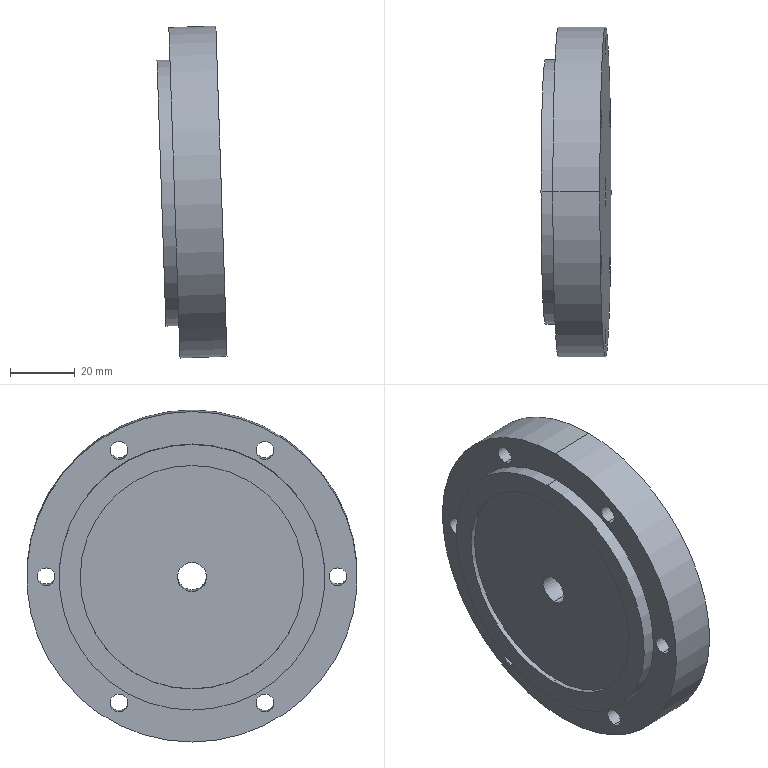Part | STEP file | 2026.6.15-Main Assembly图.sldasm-Part-80 | 1 solid | 24 faces | box 21.6 x 102 x 102.432 mm | volume 130850 mm3 | cylinder 20 | plane 4 | commonest cylinder face diameters 5.5 x12 9 x2 69 x2 82 x2 102 x2
STEP:
#1=CARTESIAN_POINT('',(-1697.272,735.086,4148.952));
#2=VERTEX_POINT('',#1);
#3=CARTESIAN_POINT('',(-1694.939,735.086,4079.992));
#4=VERTEX_POINT('',#3);
#5=CARTESIAN_POINT('',(-1696.105,735.086,4114.472));
#6=DIRECTION('',(0.9994,0.,0.03381));
#7=DIRECTION('',(0.01691,0.866,-0.4997));
#8=AXIS2_PLACEMENT_3D('',#5,#6,#7);
#9=CIRCLE('',#8,34.5);
#10=EDGE_CURVE('',#2,#4,#9,.T.);
#11=ORIENTED_EDGE('',*,*,#10,.F.);
#12=CARTESIAN_POINT('',(-1695.773,735.086,4149.003));
#13=VERTEX_POINT('',#12);
#14=CARTESIAN_POINT('',(-1697.272,735.086,4148.952));
#15=DIRECTION('',(0.9994,0.,0.03381));
#16=VECTOR('',#15,1000.);
#17=LINE('',#14,#16);
#18=EDGE_CURVE('',#2,#13,#17,.T.);
#19=ORIENTED_EDGE('',*,*,#18,.T.);
#20=CARTESIAN_POINT('',(-1693.44,735.086,4080.043));
#21=VERTEX_POINT('',#20);
#22=CARTESIAN_POINT('',(-1694.606,735.086,4114.523));
#23=DIRECTION('',(0.9994,0.,0.03381));
#24=DIRECTION('',(0.01691,0.866,-0.4997));
#25=AXIS2_PLACEMENT_3D('',#22,#23,#24);
#26=CIRCLE('',#25,34.5);
#27=EDGE_CURVE('',#13,#21,#26,.T.);
#28=ORIENTED_EDGE('',*,*,#27,.T.);
#29=CARTESIAN_POINT('',(-1694.939,735.086,4079.992));
#30=DIRECTION('',(0.9994,0.,0.03381));
#31=VECTOR('',#30,1000.);
#32=LINE('',#29,#31);
#33=EDGE_CURVE('',#4,#21,#32,.T.);
#34=ORIENTED_EDGE('',*,*,#33,.F.);
#35=EDGE_LOOP('',(#11,#19,#28,#34));
#36=FACE_OUTER_BOUND('',#35,.T.);
#37=CARTESIAN_POINT('',(-1696.105,735.086,4114.472));
#38=DIRECTION('',(0.9994,0.,0.03381));
#39=DIRECTION('',(0.03381,0.,-0.9994));
#40=AXIS2_PLACEMENT_3D('',#37,#38,#39);
#41=CYLINDRICAL_SURFACE('',#40,34.5);
#42=ADVANCED_FACE('',(#36),#41,.F.);
#43=CARTESIAN_POINT('',(-1694.719,735.086,4073.496));
#44=VERTEX_POINT('',#43);
#45=CARTESIAN_POINT('',(-1697.492,735.086,4155.449));
#46=VERTEX_POINT('',#45);
#47=CARTESIAN_POINT('',(-1696.105,735.086,4114.472));
#48=DIRECTION('',(0.9994,0.,0.03381));
#49=DIRECTION('',(0.01691,0.866,-0.4997));
#50=AXIS2_PLACEMENT_3D('',#47,#48,#49);
#51=CIRCLE('',#50,41.);
#52=EDGE_CURVE('',#44,#46,#51,.T.);
#53=ORIENTED_EDGE('',*,*,#52,.T.);
#54=CARTESIAN_POINT('',(-1693.494,735.086,4155.584));
#55=VERTEX_POINT('',#54);
#56=CARTESIAN_POINT('',(-1697.492,735.086,4155.449));
#57=DIRECTION('',(0.9994,0.,0.03381));
#58=VECTOR('',#57,1000.);
#59=LINE('',#56,#58);
#60=EDGE_CURVE('',#46,#55,#59,.T.);
#61=ORIENTED_EDGE('',*,*,#60,.T.);
#62=CARTESIAN_POINT('',(-1690.721,735.086,4073.631));
#63=VERTEX_POINT('',#62);
#64=CARTESIAN_POINT('',(-1692.108,735.086,4114.607));
#65=DIRECTION('',(0.9994,0.,0.03381));
#66=DIRECTION('',(0.01691,0.866,-0.4997));
#67=AXIS2_PLACEMENT_3D('',#64,#65,#66);
#68=CIRCLE('',#67,41.);
#69=EDGE_CURVE('',#63,#55,#68,.T.);
#70=ORIENTED_EDGE('',*,*,#69,.F.);
#71=CARTESIAN_POINT('',(-1694.719,735.086,4073.496));
#72=DIRECTION('',(0.9994,0.,0.03381));
#73=VECTOR('',#72,1000.);
#74=LINE('',#71,#73);
#75=EDGE_CURVE('',#44,#63,#74,.T.);
#76=ORIENTED_EDGE('',*,*,#75,.F.);
#77=EDGE_LOOP('',(#53,#61,#70,#76));
#78=FACE_OUTER_BOUND('',#77,.T.);
#79=CARTESIAN_POINT('',(-1696.105,735.086,4114.472));
#80=DIRECTION('',(0.9994,0.,0.03381));
#81=DIRECTION('',(0.03381,0.,-0.9994));
#82=AXIS2_PLACEMENT_3D('',#79,#80,#81);
#83=CYLINDRICAL_SURFACE('',#82,41.);
#84=ADVANCED_FACE('',(#78),#83,.T.);
#85=CARTESIAN_POINT('',(-1693.518,757.586,4156.305));
#86=VERTEX_POINT('',#85);
#87=CARTESIAN_POINT('',(-1693.332,757.586,4150.808));
#88=VERTEX_POINT('',#87);
#89=CARTESIAN_POINT('',(-1693.425,757.586,4153.556));
#90=DIRECTION('',(0.9994,0.,0.03381));
#91=DIRECTION('',(-0.02928,0.5,0.8655));
#92=AXIS2_PLACEMENT_3D('',#89,#90,#91);
#93=CIRCLE('',#92,2.75);
#94=EDGE_CURVE('',#86,#88,#93,.T.);
#95=ORIENTED_EDGE('',*,*,#94,.F.);
#96=CARTESIAN_POINT('',(-1679.027,757.586,4156.795));
#97=VERTEX_POINT('',#96);
#98=CARTESIAN_POINT('',(-1696.017,757.586,4156.22));
#99=DIRECTION('',(0.9994,0.,0.03381));
#100=VECTOR('',#99,1000.);
#101=LINE('',#98,#100);
#102=EDGE_CURVE('',#86,#97,#101,.T.);
#103=ORIENTED_EDGE('',*,*,#102,.T.);
#104=CARTESIAN_POINT('',(-1678.841,757.586,4151.298));
#105=VERTEX_POINT('',#104);
#106=CARTESIAN_POINT('',(-1678.934,757.586,4154.047));
#107=DIRECTION('',(0.9994,0.,0.03381));
#108=DIRECTION('',(-0.02928,0.5,0.8655));
#109=AXIS2_PLACEMENT_3D('',#106,#107,#108);
#110=CIRCLE('',#109,2.75);
#111=EDGE_CURVE('',#97,#105,#110,.T.);
#112=ORIENTED_EDGE('',*,*,#111,.T.);
#113=CARTESIAN_POINT('',(-1695.831,757.586,4150.723));
#114=DIRECTION('',(0.9994,0.,0.03381));
#115=VECTOR('',#114,1000.);
#116=LINE('',#113,#115);
#117=EDGE_CURVE('',#88,#105,#116,.T.);
#118=ORIENTED_EDGE('',*,*,#117,.F.);
#119=EDGE_LOOP('',(#95,#103,#112,#118));
#120=FACE_OUTER_BOUND('',#119,.T.);
#121=CARTESIAN_POINT('',(-1695.924,757.586,4153.472));
#122=DIRECTION('',(0.9994,0.,0.03381));
#123=DIRECTION('',(0.03381,0.,-0.9994));
#124=AXIS2_PLACEMENT_3D('',#121,#122,#123);
#125=CYLINDRICAL_SURFACE('',#124,2.75);
#126=ADVANCED_FACE('',(#120),#125,.F.);
#127=CARTESIAN_POINT('',(-1690.383,735.086,4063.637));
#128=VERTEX_POINT('',#127);
#129=CARTESIAN_POINT('',(-1693.832,735.086,4165.578));
#130=VERTEX_POINT('',#129);
#131=CARTESIAN_POINT('',(-1692.108,735.086,4114.607));
#132=DIRECTION('',(0.9994,0.,0.03381));
#133=DIRECTION('',(-0.02928,0.5,0.8655));
#134=AXIS2_PLACEMENT_3D('',#131,#132,#133);
#135=CIRCLE('',#134,51.);
#136=EDGE_CURVE('',#128,#130,#135,.T.);
#137=ORIENTED_EDGE('',*,*,#136,.T.);
#138=CARTESIAN_POINT('',(-1679.34,735.086,4166.069));
#139=VERTEX_POINT('',#138);
#140=CARTESIAN_POINT('',(-1696.331,735.086,4165.494));
#141=DIRECTION('',(0.9994,0.,0.03381));
#142=VECTOR('',#141,1000.);
#143=LINE('',#140,#142);
#144=EDGE_CURVE('',#130,#139,#143,.T.);
#145=ORIENTED_EDGE('',*,*,#144,.T.);
#146=CARTESIAN_POINT('',(-1675.891,735.086,4064.127));
#147=VERTEX_POINT('',#146);
#148=CARTESIAN_POINT('',(-1677.616,735.086,4115.098));
#149=DIRECTION('',(0.9994,0.,0.03381));
#150=DIRECTION('',(-0.02928,0.5,0.8655));
#151=AXIS2_PLACEMENT_3D('',#148,#149,#150);
#152=CIRCLE('',#151,51.);
#153=EDGE_CURVE('',#147,#139,#152,.T.);
#154=ORIENTED_EDGE('',*,*,#153,.F.);
#155=CARTESIAN_POINT('',(-1692.882,735.086,4063.552));
#156=DIRECTION('',(0.9994,0.,0.03381));
#157=VECTOR('',#156,1000.);
#158=LINE('',#155,#157);
#159=EDGE_CURVE('',#128,#147,#158,.T.);
#160=ORIENTED_EDGE('',*,*,#159,.F.);
#161=EDGE_LOOP('',(#137,#145,#154,#160));
#162=FACE_OUTER_BOUND('',#161,.T.);
#163=CARTESIAN_POINT('',(-1694.606,735.086,4114.523));
#164=DIRECTION('',(0.9994,0.,0.03381));
#165=DIRECTION('',(0.03381,0.,-0.9994));
#166=AXIS2_PLACEMENT_3D('',#163,#164,#165);
#167=CYLINDRICAL_SURFACE('',#166,51.);
#168=ADVANCED_FACE('',(#162),#167,.T.);
#169=CARTESIAN_POINT('',(-1693.518,712.586,4156.305));
#170=VERTEX_POINT('',#169);
#171=CARTESIAN_POINT('',(-1693.332,712.586,4150.808));
#172=VERTEX_POINT('',#171);
#173=CARTESIAN_POINT('',(-1693.425,712.586,4153.556));
#174=DIRECTION('',(0.9994,0.,0.03381));
#175=DIRECTION('',(-0.02928,0.5,0.8655));
#176=AXIS2_PLACEMENT_3D('',#173,#174,#175);
#177=CIRCLE('',#176,2.75);
#178=EDGE_CURVE('',#170,#172,#177,.T.);
#179=ORIENTED_EDGE('',*,*,#178,.F.);
#180=CARTESIAN_POINT('',(-1679.027,712.586,4156.795));
#181=VERTEX_POINT('',#180);
#182=CARTESIAN_POINT('',(-1696.017,712.586,4156.22));
#183=DIRECTION('',(0.9994,0.,0.03381));
#184=VECTOR('',#183,1000.);
#185=LINE('',#182,#184);
#186=EDGE_CURVE('',#170,#181,#185,.T.);
#187=ORIENTED_EDGE('',*,*,#186,.T.);
#188=CARTESIAN_POINT('',(-1678.841,712.586,4151.298));
#189=VERTEX_POINT('',#188);
#190=CARTESIAN_POINT('',(-1678.934,712.586,4154.047));
#191=DIRECTION('',(0.9994,0.,0.03381));
#192=DIRECTION('',(-0.02928,0.5,0.8655));
#193=AXIS2_PLACEMENT_3D('',#190,#191,#192);
#194=CIRCLE('',#193,2.75);
#195=EDGE_CURVE('',#181,#189,#194,.T.);
#196=ORIENTED_EDGE('',*,*,#195,.T.);
#197=CARTESIAN_POINT('',(-1695.831,712.586,4150.723));
#198=DIRECTION('',(0.9994,0.,0.03381));
#199=VECTOR('',#198,1000.);
#200=LINE('',#197,#199);
#201=EDGE_CURVE('',#172,#189,#200,.T.);
#202=ORIENTED_EDGE('',*,*,#201,.F.);
#203=EDGE_LOOP('',(#179,#187,#196,#202));
#204=FACE_OUTER_BOUND('',#203,.T.);
#205=CARTESIAN_POINT('',(-1695.924,712.586,4153.472));
#206=DIRECTION('',(0.9994,0.,0.03381));
#207=DIRECTION('',(0.03381,0.,-0.9994));
#208=AXIS2_PLACEMENT_3D('',#205,#206,#207);
#209=CYLINDRICAL_SURFACE('',#208,2.75);
#210=ADVANCED_FACE('',(#204),#209,.F.);
#211=CARTESIAN_POINT('',(-1692.201,690.086,4117.356));
#212=VERTEX_POINT('',#211);
#213=CARTESIAN_POINT('',(-1692.015,690.086,4111.859));
#214=VERTEX_POINT('',#213);
#215=CARTESIAN_POINT('',(-1692.108,690.086,4114.607));
#216=DIRECTION('',(0.9994,0.,0.03381));
#217=DIRECTION('',(-0.02928,0.5,0.8655));
#218=AXIS2_PLACEMENT_3D('',#215,#216,#217);
#219=CIRCLE('',#218,2.75);
#220=EDGE_CURVE('',#212,#214,#219,.T.);
#221=ORIENTED_EDGE('',*,*,#220,.F.);
#222=CARTESIAN_POINT('',(-1677.709,690.086,4117.846));
#223=VERTEX_POINT('',#222);
#224=CARTESIAN_POINT('',(-1694.699,690.086,4117.271));
#225=DIRECTION('',(0.9994,0.,0.03381));
#226=VECTOR('',#225,1000.);
#227=LINE('',#224,#226);
#228=EDGE_CURVE('',#212,#223,#227,.T.);
#229=ORIENTED_EDGE('',*,*,#228,.T.);
#230=CARTESIAN_POINT('',(-1677.523,690.086,4112.349));
#231=VERTEX_POINT('',#230);
#232=CARTESIAN_POINT('',(-1677.616,690.086,4115.098));
#233=DIRECTION('',(0.9994,0.,0.03381));
#234=DIRECTION('',(-0.02928,0.5,0.8655));
#235=AXIS2_PLACEMENT_3D('',#232,#233,#234);
#236=CIRCLE('',#235,2.75);
#237=EDGE_CURVE('',#223,#231,#236,.T.);
#238=ORIENTED_EDGE('',*,*,#237,.T.);
#239=CARTESIAN_POINT('',(-1694.513,690.086,4111.774));
#240=DIRECTION('',(0.9994,0.,0.03381));
#241=VECTOR('',#240,1000.);
#242=LINE('',#239,#241);
#243=EDGE_CURVE('',#214,#231,#242,.T.);
#244=ORIENTED_EDGE('',*,*,#243,.F.);
#245=EDGE_LOOP('',(#221,#229,#238,#244));
#246=FACE_OUTER_BOUND('',#245,.T.);
#247=CARTESIAN_POINT('',(-1694.606,690.086,4114.523));
#248=DIRECTION('',(0.9994,0.,0.03381));
#249=DIRECTION('',(0.03381,0.,-0.9994));
#250=AXIS2_PLACEMENT_3D('',#247,#248,#249);
#251=CYLINDRICAL_SURFACE('',#250,2.75);
#252=ADVANCED_FACE('',(#246),#251,.F.);
#253=CARTESIAN_POINT('',(-1690.883,757.586,4078.407));
#254=VERTEX_POINT('',#253);
#255=CARTESIAN_POINT('',(-1690.697,757.586,4072.91));
#256=VERTEX_POINT('',#255);
#257=CARTESIAN_POINT('',(-1690.79,757.586,4075.659));
#258=DIRECTION('',(0.9994,0.,0.03381));
#259=DIRECTION('',(-0.02928,0.5,0.8655));
#260=AXIS2_PLACEMENT_3D('',#257,#258,#259);
#261=CIRCLE('',#260,2.75);
#262=EDGE_CURVE('',#254,#256,#261,.T.);
#263=ORIENTED_EDGE('',*,*,#262,.F.);
#264=CARTESIAN_POINT('',(-1676.391,757.586,4078.897));
#265=VERTEX_POINT('',#264);
#266=CARTESIAN_POINT('',(-1693.381,757.586,4078.322));
#267=DIRECTION('',(0.9994,0.,0.03381));
#268=VECTOR('',#267,1000.);
#269=LINE('',#266,#268);
#270=EDGE_CURVE('',#254,#265,#269,.T.);
#271=ORIENTED_EDGE('',*,*,#270,.T.);
#272=CARTESIAN_POINT('',(-1676.205,757.586,4073.4));
#273=VERTEX_POINT('',#272);
#274=CARTESIAN_POINT('',(-1676.298,757.586,4076.149));
#275=DIRECTION('',(0.9994,0.,0.03381));
#276=DIRECTION('',(-0.02928,0.5,0.8655));
#277=AXIS2_PLACEMENT_3D('',#274,#275,#276);
#278=CIRCLE('',#277,2.75);
#279=EDGE_CURVE('',#265,#273,#278,.T.);
#280=ORIENTED_EDGE('',*,*,#279,.T.);
#281=CARTESIAN_POINT('',(-1693.195,757.586,4072.826));
#282=DIRECTION('',(0.9994,0.,0.03381));
#283=VECTOR('',#282,1000.);
#284=LINE('',#281,#283);
#285=EDGE_CURVE('',#256,#273,#284,.T.);
#286=ORIENTED_EDGE('',*,*,#285,.F.);
#287=EDGE_LOOP('',(#263,#271,#280,#286));
#288=FACE_OUTER_BOUND('',#287,.T.);
#289=CARTESIAN_POINT('',(-1693.288,757.586,4075.574));
#290=DIRECTION('',(0.9994,0.,0.03381));
#291=DIRECTION('',(0.03381,0.,-0.9994));
#292=AXIS2_PLACEMENT_3D('',#289,#290,#291);
#293=CYLINDRICAL_SURFACE('',#292,2.75);
#294=ADVANCED_FACE('',(#288),#293,.F.);
#295=CARTESIAN_POINT('',(-1690.883,712.586,4078.407));
#296=VERTEX_POINT('',#295);
#297=CARTESIAN_POINT('',(-1690.697,712.586,4072.91));
#298=VERTEX_POINT('',#297);
#299=CARTESIAN_POINT('',(-1690.79,712.586,4075.659));
#300=DIRECTION('',(0.9994,0.,0.03381));
#301=DIRECTION('',(-0.02928,0.5,0.8655));
#302=AXIS2_PLACEMENT_3D('',#299,#300,#301);
#303=CIRCLE('',#302,2.75);
#304=EDGE_CURVE('',#296,#298,#303,.T.);
#305=ORIENTED_EDGE('',*,*,#304,.F.);
#306=CARTESIAN_POINT('',(-1676.391,712.586,4078.897));
#307=VERTEX_POINT('',#306);
#308=CARTESIAN_POINT('',(-1693.381,712.586,4078.322));
#309=DIRECTION('',(0.9994,0.,0.03381));
#310=VECTOR('',#309,1000.);
#311=LINE('',#308,#310);
#312=EDGE_CURVE('',#296,#307,#311,.T.);
#313=ORIENTED_EDGE('',*,*,#312,.T.);
#314=CARTESIAN_POINT('',(-1676.205,712.586,4073.4));
#315=VERTEX_POINT('',#314);
#316=CARTESIAN_POINT('',(-1676.298,712.586,4076.149));
#317=DIRECTION('',(0.9994,0.,0.03381));
#318=DIRECTION('',(-0.02928,0.5,0.8655));
#319=AXIS2_PLACEMENT_3D('',#316,#317,#318);
#320=CIRCLE('',#319,2.75);
#321=EDGE_CURVE('',#307,#315,#320,.T.);
#322=ORIENTED_EDGE('',*,*,#321,.T.);
#323=CARTESIAN_POINT('',(-1693.195,712.586,4072.826));
#324=DIRECTION('',(0.9994,0.,0.03381));
#325=VECTOR('',#324,1000.);
#326=LINE('',#323,#325);
#327=EDGE_CURVE('',#298,#315,#326,.T.);
#328=ORIENTED_EDGE('',*,*,#327,.F.);
#329=EDGE_LOOP('',(#305,#313,#322,#328));
#330=FACE_OUTER_BOUND('',#329,.T.);
#331=CARTESIAN_POINT('',(-1693.288,712.586,4075.574));
#332=DIRECTION('',(0.9994,0.,0.03381));
#333=DIRECTION('',(0.03381,0.,-0.9994));
#334=AXIS2_PLACEMENT_3D('',#331,#332,#333);
#335=CYLINDRICAL_SURFACE('',#334,2.75);
#336=ADVANCED_FACE('',(#330),#335,.F.);
#337=CARTESIAN_POINT('',(-1694.758,735.086,4119.02));
#338=VERTEX_POINT('',#337);
#339=CARTESIAN_POINT('',(-1694.454,735.086,4110.025));
#340=VERTEX_POINT('',#339);
#341=CARTESIAN_POINT('',(-1694.606,735.086,4114.523));
#342=DIRECTION('',(0.9994,0.,0.03381));
#343=DIRECTION('',(-0.02928,0.5,0.8655));
#344=AXIS2_PLACEMENT_3D('',#341,#342,#343);
#345=CIRCLE('',#344,4.5);
#346=EDGE_CURVE('',#338,#340,#345,.T.);
#347=ORIENTED_EDGE('',*,*,#346,.F.);
#348=CARTESIAN_POINT('',(-1677.768,735.086,4119.595));
#349=VERTEX_POINT('',#348);
#350=CARTESIAN_POINT('',(-1694.758,735.086,4119.02));
#351=DIRECTION('',(0.9994,0.,0.03381));
#352=VECTOR('',#351,1000.);
#353=LINE('',#350,#352);
#354=EDGE_CURVE('',#338,#349,#353,.T.);
#355=ORIENTED_EDGE('',*,*,#354,.T.);
#356=CARTESIAN_POINT('',(-1677.464,735.086,4110.6));
#357=VERTEX_POINT('',#356);
#358=CARTESIAN_POINT('',(-1677.616,735.086,4115.098));
#359=DIRECTION('',(0.9994,0.,0.03381));
#360=DIRECTION('',(-0.02928,0.5,0.8655));
#361=AXIS2_PLACEMENT_3D('',#358,#359,#360);
#362=CIRCLE('',#361,4.5);
#363=EDGE_CURVE('',#349,#357,#362,.T.);
#364=ORIENTED_EDGE('',*,*,#363,.T.);
#365=CARTESIAN_POINT('',(-1694.454,735.086,4110.025));
#366=DIRECTION('',(0.9994,0.,0.03381));
#367=VECTOR('',#366,1000.);
#368=LINE('',#365,#367);
#369=EDGE_CURVE('',#340,#357,#368,.T.);
#370=ORIENTED_EDGE('',*,*,#369,.F.);
#371=EDGE_LOOP('',(#347,#355,#364,#370));
#372=FACE_OUTER_BOUND('',#371,.T.);
#373=CARTESIAN_POINT('',(-1694.606,735.086,4114.523));
#374=DIRECTION('',(0.9994,0.,0.03381));
#375=DIRECTION('',(0.03381,0.,-0.9994));
#376=AXIS2_PLACEMENT_3D('',#373,#374,#375);
#377=CYLINDRICAL_SURFACE('',#376,4.5);
#378=ADVANCED_FACE('',(#372),#377,.F.);
#379=CARTESIAN_POINT('',(-1692.201,780.086,4117.356));
#380=VERTEX_POINT('',#379);
#381=CARTESIAN_POINT('',(-1692.015,780.086,4111.859));
#382=VERTEX_POINT('',#381);
#383=CARTESIAN_POINT('',(-1692.108,780.086,4114.607));
#384=DIRECTION('',(0.9994,0.,0.03381));
#385=DIRECTION('',(-0.02928,0.5,0.8655));
#386=AXIS2_PLACEMENT_3D('',#383,#384,#385);
#387=CIRCLE('',#386,2.75);
#388=EDGE_CURVE('',#380,#382,#387,.T.);
#389=ORIENTED_EDGE('',*,*,#388,.F.);
#390=CARTESIAN_POINT('',(-1677.709,780.086,4117.846));
#391=VERTEX_POINT('',#390);
#392=CARTESIAN_POINT('',(-1694.699,780.086,4117.271));
#393=DIRECTION('',(0.9994,0.,0.03381));
#394=VECTOR('',#393,1000.);
#395=LINE('',#392,#394);
#396=EDGE_CURVE('',#380,#391,#395,.T.);
#397=ORIENTED_EDGE('',*,*,#396,.T.);
#398=CARTESIAN_POINT('',(-1677.523,780.086,4112.349));
#399=VERTEX_POINT('',#398);
#400=CARTESIAN_POINT('',(-1677.616,780.086,4115.098));
#401=DIRECTION('',(0.9994,0.,0.03381));
#402=DIRECTION('',(-0.02928,0.5,0.8655));
#403=AXIS2_PLACEMENT_3D('',#400,#401,#402);
#404=CIRCLE('',#403,2.75);
#405=EDGE_CURVE('',#391,#399,#404,.T.);
#406=ORIENTED_EDGE('',*,*,#405,.T.);
#407=CARTESIAN_POINT('',(-1694.513,780.086,4111.774));
#408=DIRECTION('',(0.9994,0.,0.03381));
#409=VECTOR('',#408,1000.);
#410=LINE('',#407,#409);
#411=EDGE_CURVE('',#382,#399,#410,.T.);
#412=ORIENTED_EDGE('',*,*,#411,.F.);
#413=EDGE_LOOP('',(#389,#397,#406,#412));
#414=FACE_OUTER_BOUND('',#413,.T.);
#415=CARTESIAN_POINT('',(-1694.606,780.086,4114.523));
#416=DIRECTION('',(0.9994,0.,0.03381));
#417=DIRECTION('',(0.03381,0.,-0.9994));
#418=AXIS2_PLACEMENT_3D('',#415,#416,#417);
#419=CYLINDRICAL_SURFACE('',#418,2.75);
#420=ADVANCED_FACE('',(#414),#419,.F.);
#421=CARTESIAN_POINT('',(-1694.606,735.086,4114.523));
#422=DIRECTION('',(0.9994,0.,0.03381));
#423=DIRECTION('',(-0.02928,0.5,0.8655));
#424=AXIS2_PLACEMENT_3D('',#421,#422,#423);
#425=CIRCLE('',#424,4.5);
#426=EDGE_CURVE('',#340,#338,#425,.T.);
#427=ORIENTED_EDGE('',*,*,#426,.T.);
#428=ORIENTED_EDGE('',*,*,#346,.T.);
#429=EDGE_LOOP('',(#427,#428));
#430=FACE_BOUND('',#429,.T.);
#431=CARTESIAN_POINT('',(-1694.606,735.086,4114.523));
#432=DIRECTION('',(0.9994,0.,0.03381));
#433=DIRECTION('',(0.01691,0.866,-0.4997));
#434=AXIS2_PLACEMENT_3D('',#431,#432,#433);
#435=CIRCLE('',#434,34.5);
#436=EDGE_CURVE('',#21,#13,#435,.T.);
#437=ORIENTED_EDGE('',*,*,#436,.F.);
#438=ORIENTED_EDGE('',*,*,#27,.F.);
#439=EDGE_LOOP('',(#437,#438));
#440=FACE_OUTER_BOUND('',#439,.T.);
#441=CARTESIAN_POINT('',(-1695.265,723.836,4133.997));
#442=DIRECTION('',(-0.9994,0.,-0.03381));
#443=DIRECTION('',(-0.03381,0.,0.9994));
#444=AXIS2_PLACEMENT_3D('',#441,#442,#443);
#445=PLANE('',#444);
#446=ADVANCED_FACE('',(#430,#440),#445,.T.);
#447=ORIENTED_EDGE('',*,*,#396,.F.);
#448=CARTESIAN_POINT('',(-1692.108,780.086,4114.607));
#449=DIRECTION('',(0.9994,0.,0.03381));
#450=DIRECTION('',(-0.02928,0.5,0.8655));
#451=AXIS2_PLACEMENT_3D('',#448,#449,#450);
#452=CIRCLE('',#451,2.75);
#453=EDGE_CURVE('',#382,#380,#452,.T.);
#454=ORIENTED_EDGE('',*,*,#453,.F.);
#455=ORIENTED_EDGE('',*,*,#411,.T.);
#456=CARTESIAN_POINT('',(-1677.616,780.086,4115.098));
#457=DIRECTION('',(0.9994,0.,0.03381));
#458=DIRECTION('',(-0.02928,0.5,0.8655));
#459=AXIS2_PLACEMENT_3D('',#456,#457,#458);
#460=CIRCLE('',#459,2.75);
#461=EDGE_CURVE('',#399,#391,#460,.T.);
#462=ORIENTED_EDGE('',*,*,#461,.T.);
#463=EDGE_LOOP('',(#447,#454,#455,#462));
#464=FACE_OUTER_BOUND('',#463,.T.);
#465=CARTESIAN_POINT('',(-1694.606,780.086,4114.523));
#466=DIRECTION('',(0.9994,0.,0.03381));
#467=DIRECTION('',(0.03381,0.,-0.9994));
#468=AXIS2_PLACEMENT_3D('',#465,#466,#467);
#469=CYLINDRICAL_SURFACE('',#468,2.75);
#470=ADVANCED_FACE('',(#464),#469,.F.);
#471=ORIENTED_EDGE('',*,*,#354,.F.);
#472=ORIENTED_EDGE('',*,*,#426,.F.);
#473=ORIENTED_EDGE('',*,*,#369,.T.);
#474=CARTESIAN_POINT('',(-1677.616,735.086,4115.098));
#475=DIRECTION('',(0.9994,0.,0.03381));
#476=DIRECTION('',(-0.02928,0.5,0.8655));
#477=AXIS2_PLACEMENT_3D('',#474,#475,#476);
#478=CIRCLE('',#477,4.5);
#479=EDGE_CURVE('',#357,#349,#478,.T.);
#480=ORIENTED_EDGE('',*,*,#479,.T.);
#481=EDGE_LOOP('',(#471,#472,#473,#480));
#482=FACE_OUTER_BOUND('',#481,.T.);
#483=CARTESIAN_POINT('',(-1694.606,735.086,4114.523));
#484=DIRECTION('',(0.9994,0.,0.03381));
#485=DIRECTION('',(0.03381,0.,-0.9994));
#486=AXIS2_PLACEMENT_3D('',#483,#484,#485);
#487=CYLINDRICAL_SURFACE('',#486,4.5);
#488=ADVANCED_FACE('',(#482),#487,.F.);
#489=ORIENTED_EDGE('',*,*,#312,.F.);
#490=CARTESIAN_POINT('',(-1690.79,712.586,4075.659));
#491=DIRECTION('',(0.9994,0.,0.03381));
#492=DIRECTION('',(-0.02928,0.5,0.8655));
#493=AXIS2_PLACEMENT_3D('',#490,#491,#492);
#494=CIRCLE('',#493,2.75);
#495=EDGE_CURVE('',#298,#296,#494,.T.);
#496=ORIENTED_EDGE('',*,*,#495,.F.);
#497=ORIENTED_EDGE('',*,*,#327,.T.);
#498=CARTESIAN_POINT('',(-1676.298,712.586,4076.149));
#499=DIRECTION('',(0.9994,0.,0.03381));
#500=DIRECTION('',(-0.02928,0.5,0.8655));
#501=AXIS2_PLACEMENT_3D('',#498,#499,#500);
#502=CIRCLE('',#501,2.75);
#503=EDGE_CURVE('',#315,#307,#502,.T.);
#504=ORIENTED_EDGE('',*,*,#503,.T.);
#505=EDGE_LOOP('',(#489,#496,#497,#504));
#506=FACE_OUTER_BOUND('',#505,.T.);
#507=CARTESIAN_POINT('',(-1693.288,712.586,4075.574));
#508=DIRECTION('',(0.9994,0.,0.03381));
#509=DIRECTION('',(0.03381,0.,-0.9994));
#510=AXIS2_PLACEMENT_3D('',#507,#508,#509);
#511=CYLINDRICAL_SURFACE('',#510,2.75);
#512=ADVANCED_FACE('',(#506),#511,.F.);
#513=ORIENTED_EDGE('',*,*,#270,.F.);
#514=CARTESIAN_POINT('',(-1690.79,757.586,4075.659));
#515=DIRECTION('',(0.9994,0.,0.03381));
#516=DIRECTION('',(-0.02928,0.5,0.8655));
#517=AXIS2_PLACEMENT_3D('',#514,#515,#516);
#518=CIRCLE('',#517,2.75);
#519=EDGE_CURVE('',#256,#254,#518,.T.);
#520=ORIENTED_EDGE('',*,*,#519,.F.);
#521=ORIENTED_EDGE('',*,*,#285,.T.);
#522=CARTESIAN_POINT('',(-1676.298,757.586,4076.149));
#523=DIRECTION('',(0.9994,0.,0.03381));
#524=DIRECTION('',(-0.02928,0.5,0.8655));
#525=AXIS2_PLACEMENT_3D('',#522,#523,#524);
#526=CIRCLE('',#525,2.75);
#527=EDGE_CURVE('',#273,#265,#526,.T.);
#528=ORIENTED_EDGE('',*,*,#527,.T.);
#529=EDGE_LOOP('',(#513,#520,#521,#528));
#530=FACE_OUTER_BOUND('',#529,.T.);
#531=CARTESIAN_POINT('',(-1693.288,757.586,4075.574));
#532=DIRECTION('',(0.9994,0.,0.03381));
#533=DIRECTION('',(0.03381,0.,-0.9994));
#534=AXIS2_PLACEMENT_3D('',#531,#532,#533);
#535=CYLINDRICAL_SURFACE('',#534,2.75);
#536=ADVANCED_FACE('',(#530),#535,.F.);
#537=ORIENTED_EDGE('',*,*,#228,.F.);
#538=CARTESIAN_POINT('',(-1692.108,690.086,4114.607));
#539=DIRECTION('',(0.9994,0.,0.03381));
#540=DIRECTION('',(-0.02928,0.5,0.8655));
#541=AXIS2_PLACEMENT_3D('',#538,#539,#540);
#542=CIRCLE('',#541,2.75);
#543=EDGE_CURVE('',#214,#212,#542,.T.);
#544=ORIENTED_EDGE('',*,*,#543,.F.);
#545=ORIENTED_EDGE('',*,*,#243,.T.);
#546=CARTESIAN_POINT('',(-1677.616,690.086,4115.098));
#547=DIRECTION('',(0.9994,0.,0.03381));
#548=DIRECTION('',(-0.02928,0.5,0.8655));
#549=AXIS2_PLACEMENT_3D('',#546,#547,#548);
#550=CIRCLE('',#549,2.75);
#551=EDGE_CURVE('',#231,#223,#550,.T.);
#552=ORIENTED_EDGE('',*,*,#551,.T.);
#553=EDGE_LOOP('',(#537,#544,#545,#552));
#554=FACE_OUTER_BOUND('',#553,.T.);
#555=CARTESIAN_POINT('',(-1694.606,690.086,4114.523));
#556=DIRECTION('',(0.9994,0.,0.03381));
#557=DIRECTION('',(0.03381,0.,-0.9994));
#558=AXIS2_PLACEMENT_3D('',#555,#556,#557);
#559=CYLINDRICAL_SURFACE('',#558,2.75);
#560=ADVANCED_FACE('',(#554),#559,.F.);
#561=ORIENTED_EDGE('',*,*,#186,.F.);
#562=CARTESIAN_POINT('',(-1693.425,712.586,4153.556));
#563=DIRECTION('',(0.9994,0.,0.03381));
#564=DIRECTION('',(-0.02928,0.5,0.8655));
#565=AXIS2_PLACEMENT_3D('',#562,#563,#564);
#566=CIRCLE('',#565,2.75);
#567=EDGE_CURVE('',#172,#170,#566,.T.);
#568=ORIENTED_EDGE('',*,*,#567,.F.);
#569=ORIENTED_EDGE('',*,*,#201,.T.);
#570=CARTESIAN_POINT('',(-1678.934,712.586,4154.047));
#571=DIRECTION('',(0.9994,0.,0.03381));
#572=DIRECTION('',(-0.02928,0.5,0.8655));
#573=AXIS2_PLACEMENT_3D('',#570,#571,#572);
#574=CIRCLE('',#573,2.75);
#575=EDGE_CURVE('',#189,#181,#574,.T.);
#576=ORIENTED_EDGE('',*,*,#575,.T.);
#577=EDGE_LOOP('',(#561,#568,#569,#576));
#578=FACE_OUTER_BOUND('',#577,.T.);
#579=CARTESIAN_POINT('',(-1695.924,712.586,4153.472));
#580=DIRECTION('',(0.9994,0.,0.03381));
#581=DIRECTION('',(0.03381,0.,-0.9994));
#582=AXIS2_PLACEMENT_3D('',#579,#580,#581);
#583=CYLINDRICAL_SURFACE('',#582,2.75);
#584=ADVANCED_FACE('',(#578),#583,.F.);
#585=ORIENTED_EDGE('',*,*,#144,.F.);
#586=CARTESIAN_POINT('',(-1692.108,735.086,4114.607));
#587=DIRECTION('',(0.9994,0.,0.03381));
#588=DIRECTION('',(-0.02928,0.5,0.8655));
#589=AXIS2_PLACEMENT_3D('',#586,#587,#588);
#590=CIRCLE('',#589,51.);
#591=EDGE_CURVE('',#130,#128,#590,.T.);
#592=ORIENTED_EDGE('',*,*,#591,.T.);
#593=ORIENTED_EDGE('',*,*,#159,.T.);
#594=CARTESIAN_POINT('',(-1677.616,735.086,4115.098));
#595=DIRECTION('',(0.9994,0.,0.03381));
#596=DIRECTION('',(-0.02928,0.5,0.8655));
#597=AXIS2_PLACEMENT_3D('',#594,#595,#596);
#598=CIRCLE('',#597,51.);
#599=EDGE_CURVE('',#139,#147,#598,.T.);
#600=ORIENTED_EDGE('',*,*,#599,.F.);
#601=EDGE_LOOP('',(#585,#592,#593,#600));
#602=FACE_OUTER_BOUND('',#601,.T.);
#603=CARTESIAN_POINT('',(-1694.606,735.086,4114.523));
#604=DIRECTION('',(0.9994,0.,0.03381));
#605=DIRECTION('',(0.03381,0.,-0.9994));
#606=AXIS2_PLACEMENT_3D('',#603,#604,#605);
#607=CYLINDRICAL_SURFACE('',#606,51.);
#608=ADVANCED_FACE('',(#602),#607,.T.);
#609=ORIENTED_EDGE('',*,*,#102,.F.);
#610=CARTESIAN_POINT('',(-1693.425,757.586,4153.556));
#611=DIRECTION('',(0.9994,0.,0.03381));
#612=DIRECTION('',(-0.02928,0.5,0.8655));
#613=AXIS2_PLACEMENT_3D('',#610,#611,#612);
#614=CIRCLE('',#613,2.75);
#615=EDGE_CURVE('',#88,#86,#614,.T.);
#616=ORIENTED_EDGE('',*,*,#615,.F.);
#617=ORIENTED_EDGE('',*,*,#117,.T.);
#618=CARTESIAN_POINT('',(-1678.934,757.586,4154.047));
#619=DIRECTION('',(0.9994,0.,0.03381));
#620=DIRECTION('',(-0.02928,0.5,0.8655));
#621=AXIS2_PLACEMENT_3D('',#618,#619,#620);
#622=CIRCLE('',#621,2.75);
#623=EDGE_CURVE('',#105,#97,#622,.T.);
#624=ORIENTED_EDGE('',*,*,#623,.T.);
#625=EDGE_LOOP('',(#609,#616,#617,#624));
#626=FACE_OUTER_BOUND('',#625,.T.);
#627=CARTESIAN_POINT('',(-1695.924,757.586,4153.472));
#628=DIRECTION('',(0.9994,0.,0.03381));
#629=DIRECTION('',(0.03381,0.,-0.9994));
#630=AXIS2_PLACEMENT_3D('',#627,#628,#629);
#631=CYLINDRICAL_SURFACE('',#630,2.75);
#632=ADVANCED_FACE('',(#626),#631,.F.);
#633=ORIENTED_EDGE('',*,*,#69,.T.);
#634=CARTESIAN_POINT('',(-1692.108,735.086,4114.607));
#635=DIRECTION('',(0.9994,0.,0.03381));
#636=DIRECTION('',(0.01691,0.866,-0.4997));
#637=AXIS2_PLACEMENT_3D('',#634,#635,#636);
#638=CIRCLE('',#637,41.);
#639=EDGE_CURVE('',#55,#63,#638,.T.);
#640=ORIENTED_EDGE('',*,*,#639,.T.);
#641=EDGE_LOOP('',(#633,#640));
#642=FACE_BOUND('',#641,.T.);
#643=ORIENTED_EDGE('',*,*,#136,.F.);
#644=ORIENTED_EDGE('',*,*,#591,.F.);
#645=EDGE_LOOP('',(#643,#644));
#646=FACE_OUTER_BOUND('',#645,.T.);
#647=ORIENTED_EDGE('',*,*,#567,.T.);
#648=ORIENTED_EDGE('',*,*,#178,.T.);
#649=EDGE_LOOP('',(#647,#648));
#650=FACE_BOUND('',#649,.T.);
#651=ORIENTED_EDGE('',*,*,#543,.T.);
#652=ORIENTED_EDGE('',*,*,#220,.T.);
#653=EDGE_LOOP('',(#651,#652));
#654=FACE_BOUND('',#653,.T.);
#655=ORIENTED_EDGE('',*,*,#519,.T.);
#656=ORIENTED_EDGE('',*,*,#262,.T.);
#657=EDGE_LOOP('',(#655,#656));
#658=FACE_BOUND('',#657,.T.);
#659=ORIENTED_EDGE('',*,*,#495,.T.);
#660=ORIENTED_EDGE('',*,*,#304,.T.);
#661=EDGE_LOOP('',(#659,#660));
#662=FACE_BOUND('',#661,.T.);
#663=ORIENTED_EDGE('',*,*,#453,.T.);
#664=ORIENTED_EDGE('',*,*,#388,.T.);
#665=EDGE_LOOP('',(#663,#664));
#666=FACE_BOUND('',#665,.T.);
#667=ORIENTED_EDGE('',*,*,#615,.T.);
#668=ORIENTED_EDGE('',*,*,#94,.T.);
#669=EDGE_LOOP('',(#667,#668));
#670=FACE_BOUND('',#669,.T.);
#671=CARTESIAN_POINT('',(-1692.767,723.836,4134.082));
#672=DIRECTION('',(-0.9994,0.,-0.03381));
#673=DIRECTION('',(-0.03381,0.,0.9994));
#674=AXIS2_PLACEMENT_3D('',#671,#672,#673);
#675=PLANE('',#674);
#676=ADVANCED_FACE('',(#642,#646,#650,#654,#658,#662,#666,#670),#675,.T.);
#677=ORIENTED_EDGE('',*,*,#153,.T.);
#678=ORIENTED_EDGE('',*,*,#599,.T.);
#679=EDGE_LOOP('',(#677,#678));
#680=FACE_OUTER_BOUND('',#679,.T.);
#681=ORIENTED_EDGE('',*,*,#575,.F.);
#682=ORIENTED_EDGE('',*,*,#195,.F.);
#683=EDGE_LOOP('',(#681,#682));
#684=FACE_BOUND('',#683,.T.);
#685=ORIENTED_EDGE('',*,*,#551,.F.);
#686=ORIENTED_EDGE('',*,*,#237,.F.);
#687=EDGE_LOOP('',(#685,#686));
#688=FACE_BOUND('',#687,.T.);
#689=ORIENTED_EDGE('',*,*,#527,.F.);
#690=ORIENTED_EDGE('',*,*,#279,.F.);
#691=EDGE_LOOP('',(#689,#690));
#692=FACE_BOUND('',#691,.T.);
#693=ORIENTED_EDGE('',*,*,#503,.F.);
#694=ORIENTED_EDGE('',*,*,#321,.F.);
#695=EDGE_LOOP('',(#693,#694));
#696=FACE_BOUND('',#695,.T.);
#697=ORIENTED_EDGE('',*,*,#479,.F.);
#698=ORIENTED_EDGE('',*,*,#363,.F.);
#699=EDGE_LOOP('',(#697,#698));
#700=FACE_BOUND('',#699,.T.);
#701=ORIENTED_EDGE('',*,*,#461,.F.);
#702=ORIENTED_EDGE('',*,*,#405,.F.);
#703=EDGE_LOOP('',(#701,#702));
#704=FACE_BOUND('',#703,.T.);
#705=ORIENTED_EDGE('',*,*,#623,.F.);
#706=ORIENTED_EDGE('',*,*,#111,.F.);
#707=EDGE_LOOP('',(#705,#706));
#708=FACE_BOUND('',#707,.T.);
#709=CARTESIAN_POINT('',(-1678.275,723.836,4134.572));
#710=DIRECTION('',(-0.9994,0.,-0.03381));
#711=DIRECTION('',(-0.03381,0.,0.9994));
#712=AXIS2_PLACEMENT_3D('',#709,#710,#711);
#713=PLANE('',#712);
#714=ADVANCED_FACE('',(#680,#684,#688,#692,#696,#700,#704,#708),#713,.F.);
#715=ORIENTED_EDGE('',*,*,#60,.F.);
#716=CARTESIAN_POINT('',(-1696.105,735.086,4114.472));
#717=DIRECTION('',(0.9994,0.,0.03381));
#718=DIRECTION('',(0.01691,0.866,-0.4997));
#719=AXIS2_PLACEMENT_3D('',#716,#717,#718);
#720=CIRCLE('',#719,41.);
#721=EDGE_CURVE('',#46,#44,#720,.T.);
#722=ORIENTED_EDGE('',*,*,#721,.T.);
#723=ORIENTED_EDGE('',*,*,#75,.T.);
#724=ORIENTED_EDGE('',*,*,#639,.F.);
#725=EDGE_LOOP('',(#715,#722,#723,#724));
#726=FACE_OUTER_BOUND('',#725,.T.);
#727=CARTESIAN_POINT('',(-1696.105,735.086,4114.472));
#728=DIRECTION('',(0.9994,0.,0.03381));
#729=DIRECTION('',(0.03381,0.,-0.9994));
#730=AXIS2_PLACEMENT_3D('',#727,#728,#729);
#731=CYLINDRICAL_SURFACE('',#730,41.);
#732=ADVANCED_FACE('',(#726),#731,.T.);
#733=ORIENTED_EDGE('',*,*,#18,.F.);
#734=CARTESIAN_POINT('',(-1696.105,735.086,4114.472));
#735=DIRECTION('',(0.9994,0.,0.03381));
#736=DIRECTION('',(0.01691,0.866,-0.4997));
#737=AXIS2_PLACEMENT_3D('',#734,#735,#736);
#738=CIRCLE('',#737,34.5);
#739=EDGE_CURVE('',#4,#2,#738,.T.);
#740=ORIENTED_EDGE('',*,*,#739,.F.);
#741=ORIENTED_EDGE('',*,*,#33,.T.);
#742=ORIENTED_EDGE('',*,*,#436,.T.);
#743=EDGE_LOOP('',(#733,#740,#741,#742));
#744=FACE_OUTER_BOUND('',#743,.T.);
#745=CARTESIAN_POINT('',(-1696.105,735.086,4114.472));
#746=DIRECTION('',(0.9994,0.,0.03381));
#747=DIRECTION('',(0.03381,0.,-0.9994));
#748=AXIS2_PLACEMENT_3D('',#745,#746,#747);
#749=CYLINDRICAL_SURFACE('',#748,34.5);
#750=ADVANCED_FACE('',(#744),#749,.F.);
#751=ORIENTED_EDGE('',*,*,#52,.F.);
#752=ORIENTED_EDGE('',*,*,#721,.F.);
#753=EDGE_LOOP('',(#751,#752));
#754=FACE_OUTER_BOUND('',#753,.T.);
#755=ORIENTED_EDGE('',*,*,#739,.T.);
#756=ORIENTED_EDGE('',*,*,#10,.T.);
#757=EDGE_LOOP('',(#755,#756));
#758=FACE_BOUND('',#757,.T.);
#759=CARTESIAN_POINT('',(-1696.105,735.086,4114.472));
#760=DIRECTION('',(-0.9994,0.,-0.03381));
#761=DIRECTION('',(-0.03381,0.,0.9994));
#762=AXIS2_PLACEMENT_3D('',#759,#760,#761);
#763=PLANE('',#762);
#764=ADVANCED_FACE('',(#754,#758),#763,.T.);
#765=CLOSED_SHELL('',(#42,#84,#126,#168,#210,#252,#294,#336,#378,#420,#446,#470,#488,#512,#536,#560,#584,#608,#632,#676,#714,#732,#750,#764));
#766=MANIFOLD_SOLID_BREP('',#765);
#767=CARTESIAN_POINT('',(0.,0.,0.));
#768=DIRECTION('',(0.,0.,1.));
#769=DIRECTION('',(1.,0.,0.));
#770=AXIS2_PLACEMENT_3D('',#767,#768,#769);
#771=(LENGTH_UNIT()NAMED_UNIT(*)SI_UNIT(.MILLI.,.METRE.));
#772=UNCERTAINTY_MEASURE_WITH_UNIT(LENGTH_MEASURE(0.00001),#771,'','');
#773=(NAMED_UNIT(*)PLANE_ANGLE_UNIT()SI_UNIT($,.RADIAN.));
#774=(NAMED_UNIT(*)SI_UNIT($,.STERADIAN.)SOLID_ANGLE_UNIT());
#775=(GEOMETRIC_REPRESENTATION_CONTEXT(3)GLOBAL_UNCERTAINTY_ASSIGNED_CONTEXT((#772))GLOBAL_UNIT_ASSIGNED_CONTEXT((#771,#773,#774))REPRESENTATION_CONTEXT('',''));
#776=ADVANCED_BREP_SHAPE_REPRESENTATION('',(#766,#770),#775);